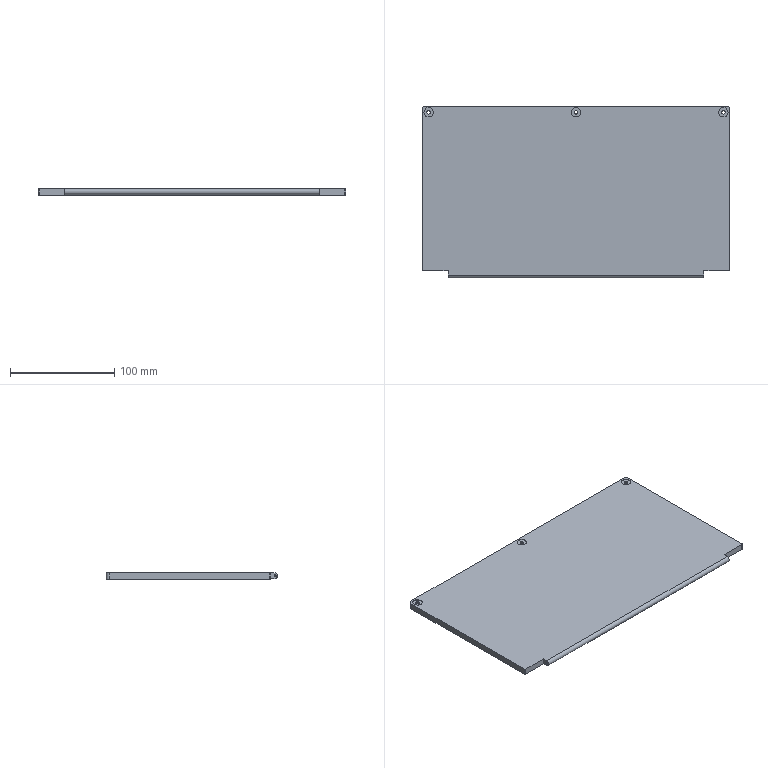NC program | Mastercam | posted with a generic post
Lines 868 to 1870 of 5159:
N8670 T6 M6
N8680 G0 G90 G17 G54 X-57.409 Y78.94 A0. S7000 M3
N8690 G43 H6 Z50. M8
N8700 Z1.
N8710 G1 Z.225 F600.
N8720 X-54.109 Z.123 F3000.
N8730 X-50.809 Z.021
N8740 X-47.509 Z-.08
N8750 X-44.209 Z-.182
N8760 X-40.909 Z-.284
N8770 X-37.609 Z-.386
N8780 X-32.744 Z-.487
N8790 G2 X-32.455 Y79.06 I27.577 J-66.293
N8800 G1 X-34.311
N8810 X-50.628
N8820 X-68.56
N8830 Y78.94
N8840 X-32.744
N8850 G2 X-32.455 Y79.06 I27.577 J-66.293
N8860 G1 X-34.311
N8870 G2 X-34.897 Y79.479 I0. J.618
N8880 G1 X-35.581 Y81.494
N8890 G3 X-36.167 Y81.913 I-.586 J-.2
N8900 G1 X-50.628
N8910 X-71.413
N8920 Y76.087
N8930 X-32.168
N8940 G2 X-7.749 Y81.913 I30.414 J-73.385
N8950 G1 X-36.167
N8960 G0 Z50.
N8970 X57.411 Y79.06
N8980 Z1.
N8990 G1 Z.225 F600.
N9000 X54.111 Z.123 F3000.
N9010 X50.811 Z.021
N9020 X47.511 Z-.08
N9030 X44.211 Z-.182
N9040 X40.911 Z-.284
N9050 X37.611 Z-.386
N9060 X32.455 Z-.487
N9070 X34.311 Y79.048
N9080 X50.628 Y78.94
N9090 X68.56
N9100 Y79.06
N9110 X32.455
N9120 X34.311 Y79.048
N9130 X34.315
N9140 G3 X34.933 Y79.666 I0. J.618
N9150 X34.723 Y80.132 I-.618 J0.
N9160 G1 X32.862 Y81.76
N9170 G3 X32.455 Y81.913 I-.407 J-.466
N9180 G1 X7.749
N9190 G2 X32.168 Y76.087 I-5.995 J-79.211
N9200 G1 X50.628
N9210 X71.413
N9220 Y81.913
N9230 X32.455
N9240 G2 X31.881 Y82.3 I0. J.619
N9250 G1 X31.172 Y84.056
N9260 G3 X30.599 Y84.443 I-.573 J-.232
N9270 G1 X0.
N9280 X-73.943
N9290 Y73.557
N9300 X-31.647
N9310 G2 X-1.474 Y79.656 I30.173 J-71.581
N9320 X2.458 Y79.557 I0. J-77.68
N9330 X31.647 Y73.557 I-.115 J-74.561
N9340 G1 X73.943
N9350 Y84.443
N9360 X30.599
N9370 G2 X29.994 Y84.928 I0. J.619
N9380 G1 X29.347 Y87.865
N9390 G3 X28.742 Y88.35 I-.605 J-.134
N9400 G1 X0.
N9410 X-77.85
N9420 Y69.65
N9430 X-30.822
N9440 G2 X-1.437 Y75.753 I29.385 J-67.691
N9450 X2.458 Y75.65 I0. J-73.794
N9460 X30.822 Y69.65 I-.108 J-70.552
N9470 G1 X77.85
N9480 Y88.35
N9490 X28.742
N9500 G2 X28.138 Y88.835 I0. J.619
N9510 G1 X27.49 Y91.772
N9520 G3 X26.886 Y92.257 I-.604 J-.134
N9530 G1 X0.
N9540 X-81.757
N9550 Y65.743
N9560 X-29.97
N9570 G2 X-1.396 Y71.849 I28.574 J-63.801
N9580 X2.458 Y71.743 I0. J-69.907
N9590 X29.97 Y65.743 I-.099 J-66.53
N9600 G1 X81.757
N9610 Y92.257
N9620 X26.886
N9630 G2 X26.282 Y92.742 I0. J.619
N9640 G1 X25.634 Y95.678
N9650 G3 X25.03 Y96.164 I-.604 J-.133
N9660 G1 X0.
N9670 X-85.664
N9680 Y61.836
N9690 X-29.088
N9700 G2 X-1.371 Y67.948 I27.717 J-59.793
N9710 X2.458 Y67.836 I0. J-65.905
N9720 X29.088 Y61.836 I-.089 J-62.489
N9730 G1 X85.664
N9740 Y96.164
N9750 X25.03
N9760 G2 X24.426 Y96.649 I0. J.618
N9770 G1 X23.778 Y99.585
N9780 G3 X23.174 Y100.07 I-.604 J-.133
N9790 G1 X0.
N9800 X-89.57
N9810 Y57.93
N9820 X-28.171
N9830 G2 X-1.357 Y64.048 I26.814 J-55.705
N9840 X2.458 Y63.93 I0. J-61.823
N9850 X28.171 Y57.93 I-.044 J-58.289
N9860 G1 X89.57
N9870 Y100.07
N9880 X23.174
N9890 G2 X22.569 Y100.556 I0. J.619
N9900 G1 X21.922 Y103.492
N9910 G3 X21.317 Y103.977 I-.605 J-.133
N9920 G1 X0.
N9930 X-93.477
N9940 Y54.023
N9950 X-27.222
N9960 G2 X-1.331 Y60.148 I25.891 J-51.663
N9970 X2.458 Y60.023 I0. J-57.788
N9980 X27.222 Y54.023 I-.007 J-54.13
N9990 G1 X93.477
N100 Y103.977
N110 X21.317
N120 G2 X20.713 Y104.463 I0. J.619
N130 G1 X20.065 Y107.399
N140 G3 X19.461 Y107.884 I-.604 J-.134
N150 G1 X0.
N160 X-97.384
N170 Y50.116
N180 X-26.251
N190 G2 X-1.291 Y56.246 I24.96 J-47.748
N200 X2.458 Y56.116 I0. J-53.878
N210 G1 X2.463
N220 G2 X26.251 Y50.116 I0. J-50.159
N230 G1 X97.384
N240 Y107.884
N250 X19.461
N260 G2 X18.857 Y108.369 I0. J.619
N270 G1 X18.209 Y111.306
N280 G3 X17.605 Y111.791 I-.604 J-.134
N290 G1 X0.
N300 X-101.291
N310 Y46.209
N320 X-25.233
N330 G2 X-1.247 Y52.346 I23.986 J-43.802
N340 X2.458 Y52.209 I0. J-49.939
N350 G1 X2.479
N360 G2 X25.233 Y46.209 I0. J-46.148
N370 G1 X101.291
N380 Y111.791
N390 X17.605
N400 G2 X17.001 Y112.276 I0. J.619
N410 G1 X16.353 Y115.212
N420 G3 X15.749 Y115.698 I-.604 J-.133
N430 G1 X0.
N440 X-105.198
N450 Y42.302
N460 X-24.182
N470 G2 X-1.192 Y48.447 I22.99 J-39.935
N480 X2.458 Y48.302 I0. J-46.08
N490 G1 X2.476
N500 G2 X24.182 Y42.302 I0. J-42.263
N510 G1 X105.198
N520 Y115.698
N530 X15.749
N540 G2 X15.144 Y116.183 I0. J.619
N550 G1 X14.497 Y119.119
N560 G3 X13.892 Y119.605 I-.605 J-.133
N570 G1 X0.
N580 X-109.105
N590 Y38.395
N600 X-23.072
N610 G2 X-1.134 Y44.548 I21.938 J-36.03
N620 X2.458 Y44.395 I0. J-42.183
N630 G1 X2.476
N640 G2 X23.072 Y38.395 I0. J-38.347
N650 G1 X109.105
N660 Y119.605
N670 X13.892
N680 G2 X13.288 Y120.09 I0. J.618
N690 G1 X12.64 Y123.026
N700 G3 X12.036 Y123.512 I-.604 J-.133
N710 G1 X0.
N720 X-113.012
N730 Y34.488
N740 X-21.883
N750 G2 X-2.16 Y40.554 I19.723 J-29.028
N760 X0. Y40.488 I0. J-35.094
N770 X2.16 Y40.555 I2.16 J-35.028
N780 X21.883 Y34.488 I0. J-35.095
N790 G1 X113.012
N800 Y123.512
N810 X12.036
N820 G2 X11.432 Y123.997 I0. J.618
N830 G1 X10.784 Y126.933
N840 G3 X10.18 Y127.419 I-.604 J-.133
N850 G1 X0.
N860 X-116.919
N870 Y30.581
N880 X-20.606
N890 G2 X-1.052 Y36.763 I19.554 J-27.836
N900 X2.458 Y36.581 I0. J-34.018
N910 G1 X2.521
N920 G2 X20.606 Y30.581 I0. J-30.256
N930 G1 X116.919
N940 Y127.419
N950 X10.18
N960 G2 X9.576 Y127.904 I0. J.618
N970 G1 X8.928 Y130.84
N980 G3 X8.324 Y131.325 I-.604 J-.133
N990 G1 X0.
N1000 X-120.825
N1010 Y26.675
N1020 X-19.231
N1030 G2 X-9.646 Y31.72 I18.178 J-22.906
N1040 X.06 Y32.736 I9.706 J-45.863
N1050 X2.458 Y32.675 I0. J-46.879
N1060 G1 X2.569
N1070 G2 X19.231 Y26.675 I0. J-26.136
N1080 G1 X120.825
N1090 Y131.325
N1100 X8.324
N1110 G2 X7.719 Y131.811 I0. J.619
N1120 G1 X7.072 Y134.747
N1130 G3 X6.467 Y135.232 I-.605 J-.133
N1140 G1 X0.
N1150 X-124.732
N1160 Y22.768
N1170 X-17.749
N1180 G2 X-9.083 Y27.812 I16.408 J-18.221
N1190 X.033 Y28.839 I9.116 J-39.926
N1200 X2.458 Y28.768 I0. J-40.953
N1210 G1 X2.602
N1220 G2 X17.749 Y22.768 I0. J-22.118
N1230 G1 X124.732
N1240 Y135.232
N1250 X6.467
N1260 G2 X5.863 Y135.718 I0. J.619
N1270 G1 X5.215 Y138.654
N1280 G3 X4.611 Y139.139 I-.604 J-.133
N1290 G1 X0.
N1300 X-128.639
N1310 Y20.156
N1320 X-127.344 Y18.861
N1330 X-16.156
N1340 G2 X-8.479 Y23.904 I14.872 J-14.274
N1350 X.017 Y24.946 I8.496 J-34.117
N1360 X2.458 Y24.861 I0. J-35.159
N1370 G1 X2.569
N1380 G2 X16.156 Y18.861 I0. J-18.382
N1390 G1 X127.344
N1400 X128.639 Y20.156
N1410 Y139.139
N1420 X4.611
N1430 G2 X4.007 Y139.625 I0. J.619
N1440 G1 X3.359 Y142.561
N1450 G3 X2.755 Y143.046 I-.604 J-.134
N1460 G1 X0.
N1470 X-132.546
N1480 Y18.537
N1490 X-128.963 Y14.954
N1500 X-14.537
N1510 G2 X-7.724 Y20.031 I15.103 J-13.158
N1520 X.111 Y21.055 I7.835 J-29.465
N1530 X2.604 Y20.953 I0. J-30.489
N1540 X14.537 Y14.954 I-.387 J-15.639
N1550 G1 X128.963
N1560 X132.546 Y18.537
N1570 Y143.046
N1580 X2.755
N1590 G2 X2.151 Y143.532 I0. J.619
N1600 G1 X1.503 Y146.468
N1610 G3 X.899 Y146.953 I-.604 J-.134
N1620 G1 X0.
N1630 X-136.453
N1640 Y16.919
N1650 X-130.581 Y11.047
N1660 X-12.919
N1670 G2 X-6.446 Y16.339 I16.004 J-12.971
N1680 X.1 Y17.151 I6.546 J-25.972
N1690 X2.458 Y17.047 I0. J-26.784
N1700 X7.68 Y15.742 I-.48 J-13.021
N1710 X12.919 Y11.047 I-12.589 J-19.319
N1720 G1 X130.581
N1730 X136.453 Y16.919
N1740 Y146.953
N1750 X.899
N1760 G2 X.28 Y147.572 I0. J.619
N1770 X.285 Y147.652 I.619 J0.
N1780 G1 X.614 Y150.161
N1790 G3 X.619 Y150.241 I-.614 J.08
N1800 X0. Y150.86 I-.619 J0.
N1810 G1 X-140.244
N1820 X-140.353 Y150.853
N1830 X-140.36 Y150.268
N1840 Y15.924
N1850 X-140.343 Y15.309
N1860 X-140.261 Y15.202
N1870 X-132.474 Y7.414
N1880 X-132.193 Y7.158
N1890 X-132.081 Y7.143
N1900 X-131.927 Y7.14
N1910 X-11.506
N1920 X-11.309 Y7.157
N1930 X-11.199 Y7.242
N1940 X-6.862 Y11.555
N1950 G2 X-5.167 Y12.647 I4.319 J-4.842
N1960 X-3.005 Y13.13 I2.491 J-6.075
N1970 X.043 Y13.157 I3.048 J-169.278
N1980 X2.458 Y13.14 I0. J-169.305
N1990 X2.676 Y13.144 I.218 J-6.388
N2000 X6.175 Y12.101 I0. J-6.392
N2010 X7.375 Y11.066 I-7.862 J-10.326
N2020 G1 X11.199 Y7.242
N2030 X11.309 Y7.157
N2040 X11.506 Y7.14
N2050 X131.927
N2060 X132.193 Y7.158
N2070 X132.474 Y7.414
N2080 X140.261 Y15.202
N2090 X140.342 Y15.307
N2100 X140.352 Y15.378
N2110 X140.36 Y150.268
N2120 X140.354 Y150.85
N2130 X140.244 Y150.86
N2140 X0.
N2150 G0 Z50.
N2160 X-57.409 Y78.94
N2170 Z.512
N2180 G1 Z-.263 F600.
N2190 X-54.109 Z-.364 F3000.
N2200 X-50.809 Z-.466
N2210 X-47.509 Z-.568
N2220 X-44.209 Z-.67
N2230 X-40.909 Z-.771
N2240 X-37.609 Z-.873
N2250 X-32.744 Z-.975
N2260 G2 X-32.455 Y79.06 I27.577 J-66.293
N2270 G1 X-34.311
N2280 X-50.628
N2290 X-68.56
N2300 Y78.94
N2310 X-32.744
N2320 G2 X-32.455 Y79.06 I27.577 J-66.293
N2330 G1 X-34.311
N2340 G2 X-34.897 Y79.479 I0. J.618
N2350 G1 X-35.581 Y81.494
N2360 G3 X-36.167 Y81.913 I-.586 J-.2
N2370 G1 X-50.628
N2380 X-71.413
N2390 Y76.087
N2400 X-32.168
N2410 G2 X-7.749 Y81.913 I30.414 J-73.385
N2420 G1 X-36.167
N2430 G0 Z50.
N2440 X57.411 Y79.06
N2450 Z.512
N2460 G1 Z-.263 F600.
N2470 X54.111 Z-.364 F3000.
N2480 X50.811 Z-.466
N2490 X47.511 Z-.568
N2500 X44.211 Z-.67
N2510 X40.911 Z-.771
N2520 X37.611 Z-.873
N2530 X32.455 Z-.975
N2540 X34.311 Y79.048
N2550 X50.628 Y78.94
N2560 X68.56
N2570 Y79.06
N2580 X32.455
N2590 X34.311 Y79.048
N2600 X34.315
N2610 G3 X34.933 Y79.666 I0. J.618
N2620 X34.723 Y80.132 I-.618 J0.
N2630 G1 X32.862 Y81.76
N2640 G3 X32.455 Y81.913 I-.407 J-.466
N2650 G1 X7.749
N2660 G2 X32.168 Y76.087 I-5.995 J-79.211
N2670 G1 X50.628
N2680 X71.413
N2690 Y81.913
N2700 X32.455
N2710 G2 X31.881 Y82.3 I0. J.619
N2720 G1 X31.172 Y84.056
N2730 G3 X30.599 Y84.443 I-.573 J-.232
N2740 G1 X0.
N2750 X-73.943
N2760 Y73.557
N2770 X-31.647
N2780 G2 X-1.474 Y79.656 I30.173 J-71.581
N2790 X2.458 Y79.557 I0. J-77.68
N2800 X31.647 Y73.557 I-.115 J-74.561
N2810 G1 X73.943
N2820 Y84.443
N2830 X30.599
N2840 G2 X29.994 Y84.928 I0. J.619
N2850 G1 X29.347 Y87.865
N2860 G3 X28.742 Y88.35 I-.605 J-.134
N2870 G1 X0.
N2880 X-77.85
N2890 Y69.65
N2900 X-30.822
N2910 G2 X-1.437 Y75.753 I29.385 J-67.691
N2920 X2.458 Y75.65 I0. J-73.794
N2930 X30.822 Y69.65 I-.108 J-70.552
N2940 G1 X77.85
N2950 Y88.35
N2960 X28.742
N2970 G2 X28.138 Y88.835 I0. J.619
N2980 G1 X27.49 Y91.772
N2990 G3 X26.886 Y92.257 I-.604 J-.134
N3000 G1 X0.
N3010 X-81.757
N3020 Y65.743
N3030 X-29.97
N3040 G2 X-1.396 Y71.849 I28.574 J-63.801
N3050 X2.458 Y71.743 I0. J-69.907
N3060 X29.97 Y65.743 I-.099 J-66.53
N3070 G1 X81.757
N3080 Y92.257
N3090 X26.886
N3100 G2 X26.282 Y92.742 I0. J.619
N3110 G1 X25.634 Y95.678
N3120 G3 X25.03 Y96.164 I-.604 J-.133
N3130 G1 X0.
N3140 X-85.664
N3150 Y61.836
N3160 X-29.088
N3170 G2 X-1.371 Y67.948 I27.717 J-59.793
N3180 X2.458 Y67.836 I0. J-65.905
N3190 X29.088 Y61.836 I-.089 J-62.489
N3200 G1 X85.664
N3210 Y96.164
N3220 X25.03
N3230 G2 X24.426 Y96.649 I0. J.618
N3240 G1 X23.778 Y99.585
N3250 G3 X23.174 Y100.07 I-.604 J-.133
N3260 G1 X0.
N3270 X-89.57
N3280 Y57.93
N3290 X-28.171
N3300 G2 X-1.357 Y64.048 I26.814 J-55.705
N3310 X2.458 Y63.93 I0. J-61.823
N3320 X28.171 Y57.93 I-.044 J-58.289
N3330 G1 X89.57
N3340 Y100.07
N3350 X23.174
N3360 G2 X22.569 Y100.556 I0. J.619
N3370 G1 X21.922 Y103.492
N3380 G3 X21.317 Y103.977 I-.605 J-.133
N3390 G1 X0.
N3400 X-93.477
N3410 Y54.023
N3420 X-27.222
N3430 G2 X-1.331 Y60.148 I25.891 J-51.663
N3440 X2.458 Y60.023 I0. J-57.788
N3450 X27.222 Y54.023 I-.007 J-54.13
N3460 G1 X93.477
N3470 Y103.977
N3480 X21.317
N3490 G2 X20.713 Y104.463 I0. J.619
N3500 G1 X20.065 Y107.399
N3510 G3 X19.461 Y107.884 I-.604 J-.134
N3520 G1 X0.
N3530 X-97.384
N3540 Y50.116
N3550 X-26.251
N3560 G2 X-1.291 Y56.246 I24.96 J-47.748
N3570 X2.458 Y56.116 I0. J-53.878
N3580 G1 X2.463
N3590 G2 X26.251 Y50.116 I0. J-50.159
N3600 G1 X97.384
N3610 Y107.884
N3620 X19.461
N3630 G2 X18.857 Y108.369 I0. J.619
N3640 G1 X18.209 Y111.306
N3650 G3 X17.605 Y111.791 I-.604 J-.134
N3660 G1 X0.
N3670 X-101.291
N3680 Y46.209
N3690 X-25.233
N3700 G2 X-1.247 Y52.346 I23.986 J-43.802
N3710 X2.458 Y52.209 I0. J-49.939
N3720 G1 X2.479
N3730 G2 X25.233 Y46.209 I0. J-46.148
N3740 G1 X101.291
N3750 Y111.791
N3760 X17.605
N3770 G2 X17.001 Y112.276 I0. J.619
N3780 G1 X16.353 Y115.212
N3790 G3 X15.749 Y115.698 I-.604 J-.133
N3800 G1 X0.
N3810 X-105.198
N3820 Y42.302
N3830 X-24.182
N3840 G2 X-1.192 Y48.447 I22.99 J-39.935
N3850 X2.458 Y48.302 I0. J-46.08
N3860 G1 X2.476
N3870 G2 X24.182 Y42.302 I0. J-42.263
N3880 G1 X105.198
N3890 Y115.698
N3900 X15.749
N3910 G2 X15.144 Y116.183 I0. J.619
N3920 G1 X14.497 Y119.119
N3930 G3 X13.892 Y119.605 I-.605 J-.133
N3940 G1 X0.
N3950 X-109.105
N3960 Y38.395
N3970 X-23.072
N3980 G2 X-1.134 Y44.548 I21.938 J-36.03
N3990 X2.458 Y44.395 I0. J-42.183
N4000 G1 X2.476
N4010 G2 X23.072 Y38.395 I0. J-38.347
N4020 G1 X109.105
N4030 Y119.605
N4040 X13.892
N4050 G2 X13.288 Y120.09 I0. J.618
N4060 G1 X12.64 Y123.026
N4070 G3 X12.036 Y123.512 I-.604 J-.133
N4080 G1 X0.
N4090 X-113.012
N4100 Y34.488
N4110 X-21.883
N4120 G2 X-2.16 Y40.554 I19.723 J-29.028
N4130 X0. Y40.488 I0. J-35.094
N4140 X2.16 Y40.555 I2.16 J-35.028
N4150 X21.883 Y34.488 I0. J-35.095
N4160 G1 X113.012
N4170 Y123.512
N4180 X12.036
N4190 G2 X11.432 Y123.997 I0. J.618
N4200 G1 X10.784 Y126.933
N4210 G3 X10.18 Y127.419 I-.604 J-.133
N4220 G1 X0.
N4230 X-116.919
N4240 Y30.581
N4250 X-20.606
N4260 G2 X-1.052 Y36.763 I19.554 J-27.836
N4270 X2.458 Y36.581 I0. J-34.018
N4280 G1 X2.521
N4290 G2 X20.606 Y30.581 I0. J-30.256
N4300 G1 X116.919
N4310 Y127.419
N4320 X10.18
N4330 G2 X9.576 Y127.904 I0. J.618
N4340 G1 X8.928 Y130.84
N4350 G3 X8.324 Y131.325 I-.604 J-.133
N4360 G1 X0.
N4370 X-120.825
N4380 Y26.675
N4390 X-19.231
N4400 G2 X-9.646 Y31.72 I18.178 J-22.906
N4410 X.06 Y32.736 I9.706 J-45.863
N4420 X2.458 Y32.675 I0. J-46.879
N4430 G1 X2.569
N4440 G2 X19.231 Y26.675 I0. J-26.136
N4450 G1 X120.825
N4460 Y131.325
N4470 X8.324
N4480 G2 X7.719 Y131.811 I0. J.619
N4490 G1 X7.072 Y134.747
N4500 G3 X6.467 Y135.232 I-.605 J-.133
N4510 G1 X0.
N4520 X-124.732
N4530 Y22.768
N4540 X-17.749
N4550 G2 X-9.083 Y27.812 I16.408 J-18.221
N4560 X.033 Y28.839 I9.116 J-39.926
N4570 X2.458 Y28.768 I0. J-40.953
N4580 G1 X2.602
N4590 G2 X17.749 Y22.768 I0. J-22.118
N4600 G1 X124.732
N4610 Y135.232
N4620 X6.467
N4630 G2 X5.863 Y135.718 I0. J.619
N4640 G1 X5.215 Y138.654
N4650 G3 X4.611 Y139.139 I-.604 J-.133
N4660 G1 X0.
N4670 X-128.639
N4680 Y20.156
N4690 X-127.344 Y18.861
N4700 X-16.156
N4710 G2 X-8.479 Y23.904 I14.872 J-14.274
N4720 X.017 Y24.946 I8.496 J-34.117
N4730 X2.458 Y24.861 I0. J-35.159
N4740 G1 X2.569
N4750 G2 X16.156 Y18.861 I0. J-18.382
N4760 G1 X127.344
N4770 X128.639 Y20.156
N4780 Y139.139
N4790 X4.611
N4800 G2 X4.007 Y139.625 I0. J.619
N4810 G1 X3.359 Y142.561
N4820 G3 X2.755 Y143.046 I-.604 J-.134
N4830 G1 X0.
N4840 X-132.546
N4850 Y18.537
N4860 X-128.963 Y14.954
N4870 X-14.537
N4880 G2 X-7.724 Y20.031 I15.103 J-13.158
N4890 X.111 Y21.055 I7.835 J-29.465
N4900 X2.604 Y20.953 I0. J-30.489
N4910 X14.537 Y14.954 I-.387 J-15.639
N4920 G1 X128.963
N4930 X132.546 Y18.537
N4940 Y143.046
N4950 X2.755
N4960 G2 X2.151 Y143.532 I0. J.619
N4970 G1 X1.503 Y146.468
N4980 G3 X.899 Y146.953 I-.604 J-.134
N4990 G1 X0.
N5000 X-136.453
N5010 Y16.919
N5020 X-130.581 Y11.047
N5030 X-12.919
N5040 G2 X-6.446 Y16.339 I16.004 J-12.971
N5050 X.1 Y17.151 I6.546 J-25.972
N5060 X2.458 Y17.047 I0. J-26.784
N5070 X7.68 Y15.742 I-.48 J-13.021
N5080 X12.919 Y11.047 I-12.589 J-19.319
N5090 G1 X130.581
N5100 X136.453 Y16.919
N5110 Y146.953
N5120 X.899
N5130 G2 X.28 Y147.572 I0. J.619
N5140 X.285 Y147.652 I.619 J0.
N5150 G1 X.614 Y150.161
N5160 G3 X.619 Y150.241 I-.614 J.08
N5170 X0. Y150.86 I-.619 J0.
N5180 G1 X-140.244
N5190 X-140.353 Y150.853
N5200 X-140.36 Y150.268
N5210 Y15.924
N5220 X-140.343 Y15.309
N5230 X-140.261 Y15.202
N5240 X-132.474 Y7.414
N5250 X-132.193 Y7.158
N5260 X-132.081 Y7.143
N5270 X-131.927 Y7.14
N5280 X-11.506
N5290 X-11.309 Y7.157
N5300 X-11.199 Y7.242
N5310 X-6.862 Y11.555
N5320 G2 X-5.167 Y12.647 I4.319 J-4.842
N5330 X-3.005 Y13.13 I2.491 J-6.075
N5340 X.043 Y13.157 I3.048 J-169.278
N5350 X2.458 Y13.14 I0. J-169.305
N5360 X2.676 Y13.144 I.218 J-6.388
N5370 X6.175 Y12.101 I0. J-6.392
N5380 X7.375 Y11.066 I-7.862 J-10.326
N5390 G1 X11.199 Y7.242
N5400 X11.309 Y7.157
N5410 X11.506 Y7.14
N5420 X131.927
N5430 X132.193 Y7.158
N5440 X132.474 Y7.414
N5450 X140.261 Y15.202
N5460 X140.342 Y15.307
N5470 X140.352 Y15.378
N5480 X140.36 Y150.268
N5490 X140.354 Y150.85
N5500 X140.244 Y150.86
N5510 X0.
N5520 G0 Z50.
N5530 X-57.409 Y78.94
N5540 Z.025
N5550 G1 Z-.75 F600.
N5560 X-54.109 Z-.852 F3000.
N5570 X-50.809 Z-.954
N5580 X-47.509 Z-1.055
N5590 X-44.209 Z-1.157
N5600 X-40.909 Z-1.259
N5610 X-37.609 Z-1.361
N5620 X-32.744 Z-1.462
N5630 G2 X-32.455 Y79.06 I27.577 J-66.293
N5640 G1 X-34.311
N5650 X-50.628
N5660 X-68.56
N5670 Y78.94
N5680 X-32.744
N5690 G2 X-32.455 Y79.06 I27.577 J-66.293
N5700 G1 X-34.311
N5710 G2 X-34.897 Y79.479 I0. J.618
N5720 G1 X-35.581 Y81.494
N5730 G3 X-36.167 Y81.913 I-.586 J-.2
N5740 G1 X-50.628
N5750 X-71.413
N5760 Y76.087
N5770 X-32.168
N5780 G2 X-7.749 Y81.913 I30.414 J-73.385
N5790 G1 X-36.167
N5800 G0 Z50.
N5810 X57.411 Y79.06
N5820 Z.025
N5830 G1 Z-.75 F600.
N5840 X54.111 Z-.852 F3000.
N5850 X50.811 Z-.954
N5860 X47.511 Z-1.055
N5870 X44.211 Z-1.157
N5880 X40.911 Z-1.259
N5890 X37.611 Z-1.361
N5900 X32.455 Z-1.462
N5910 X34.311 Y79.048
N5920 X50.628 Y78.94
N5930 X68.56
N5940 Y79.06
N5950 X32.455
N5960 X34.311 Y79.048
N5970 X34.315
N5980 G3 X34.933 Y79.666 I0. J.618
N5990 X34.723 Y80.132 I-.618 J0.
N6000 G1 X32.862 Y81.76
N6010 G3 X32.455 Y81.913 I-.407 J-.466
N6020 G1 X7.749
N6030 G2 X32.168 Y76.087 I-5.995 J-79.211
N6040 G1 X50.628
N6050 X71.413
N6060 Y81.913
N6070 X32.455
N6080 G2 X31.881 Y82.3 I0. J.619
N6090 G1 X31.172 Y84.056
N6100 G3 X30.599 Y84.443 I-.573 J-.232
N6110 G1 X0.
N6120 X-73.943
N6130 Y73.557
N6140 X-31.647
N6150 G2 X-1.474 Y79.656 I30.173 J-71.581
N6160 X2.458 Y79.557 I0. J-77.68
N6170 X31.647 Y73.557 I-.115 J-74.561
N6180 G1 X73.943
N6190 Y84.443
N6200 X30.599
N6210 G2 X29.994 Y84.928 I0. J.619
N6220 G1 X29.347 Y87.865
N6230 G3 X28.742 Y88.35 I-.605 J-.134
N6240 G1 X0.
N6250 X-77.85
N6260 Y69.65
N6270 X-30.822
N6280 G2 X-1.437 Y75.753 I29.385 J-67.691
N6290 X2.458 Y75.65 I0. J-73.794
N6300 X30.822 Y69.65 I-.108 J-70.552
N6310 G1 X77.85
N6320 Y88.35
N6330 X28.742
N6340 G2 X28.138 Y88.835 I0. J.619
N6350 G1 X27.49 Y91.772
N6360 G3 X26.886 Y92.257 I-.604 J-.134
N6370 G1 X0.
N6380 X-81.757
N6390 Y65.743
N6400 X-29.97
N6410 G2 X-1.396 Y71.849 I28.574 J-63.801
N6420 X2.458 Y71.743 I0. J-69.907
N6430 X29.97 Y65.743 I-.099 J-66.53
N6440 G1 X81.757
N6450 Y92.257
N6460 X26.886
N6470 G2 X26.282 Y92.742 I0. J.619
N6480 G1 X25.634 Y95.678
N6490 G3 X25.03 Y96.164 I-.604 J-.133
N6500 G1 X0.
N6510 X-85.664
N6520 Y61.836
N6530 X-29.088
N6540 G2 X-1.371 Y67.948 I27.717 J-59.793
N6550 X2.458 Y67.836 I0. J-65.905
N6560 X29.088 Y61.836 I-.089 J-62.489
N6570 G1 X85.664
N6580 Y96.164
N6590 X25.03
N6600 G2 X24.426 Y96.649 I0. J.618
N6610 G1 X23.778 Y99.585
N6620 G3 X23.174 Y100.07 I-.604 J-.133
N6630 G1 X0.
N6640 X-89.57
N6650 Y57.93
N6660 X-28.171
N6670 G2 X-1.357 Y64.048 I26.814 J-55.705
N6680 X2.458 Y63.93 I0. J-61.823
N6690 X28.171 Y57.93 I-.044 J-58.289
N6700 G1 X89.57
N6710 Y100.07
N6720 X23.174
N6730 G2 X22.569 Y100.556 I0. J.619
N6740 G1 X21.922 Y103.492
N6750 G3 X21.317 Y103.977 I-.605 J-.133
N6760 G1 X0.
N6770 X-93.477
N6780 Y54.023
N6790 X-27.222
N6800 G2 X-1.331 Y60.148 I25.891 J-51.663
N6810 X2.458 Y60.023 I0. J-57.788
N6820 X27.222 Y54.023 I-.007 J-54.13
N6830 G1 X93.477
N6840 Y103.977
N6850 X21.317
N6860 G2 X20.713 Y104.463 I0. J.619
N6870 G1 X20.065 Y107.399
N6880 G3 X19.461 Y107.884 I-.604 J-.134
N6890 G1 X0.
N6900 X-97.384
N6910 Y50.116
N6920 X-26.251
N6930 G2 X-1.291 Y56.246 I24.96 J-47.748
N6940 X2.458 Y56.116 I0. J-53.878
N6950 G1 X2.463
N6960 G2 X26.251 Y50.116 I0. J-50.159
N6970 G1 X97.384
N6980 Y107.884
N6990 X19.461
N7000 G2 X18.857 Y108.369 I0. J.619
N7010 G1 X18.209 Y111.306
N7020 G3 X17.605 Y111.791 I-.604 J-.134
N7030 G1 X0.
N7040 X-101.291
N7050 Y46.209
N7060 X-25.233
N7070 G2 X-1.247 Y52.346 I23.986 J-43.802
N7080 X2.458 Y52.209 I0. J-49.939
N7090 G1 X2.479
N7100 G2 X25.233 Y46.209 I0. J-46.148
N7110 G1 X101.291
N7120 Y111.791
N7130 X17.605
N7140 G2 X17.001 Y112.276 I0. J.619
N7150 G1 X16.353 Y115.212
N7160 G3 X15.749 Y115.698 I-.604 J-.133
N7170 G1 X0.
N7180 X-105.198
N7190 Y42.302
N7200 X-24.182
N7210 G2 X-1.192 Y48.447 I22.99 J-39.935
N7220 X2.458 Y48.302 I0. J-46.08
N7230 G1 X2.476
N7240 G2 X24.182 Y42.302 I0. J-42.263
N7250 G1 X105.198
N7260 Y115.698
N7270 X15.749
N7280 G2 X15.144 Y116.183 I0. J.619
N7290 G1 X14.497 Y119.119
N7300 G3 X13.892 Y119.605 I-.605 J-.133
N7310 G1 X0.
N7320 X-109.105
N7330 Y38.395
N7340 X-23.072
N7350 G2 X-1.134 Y44.548 I21.938 J-36.03
N7360 X2.458 Y44.395 I0. J-42.183
N7370 G1 X2.476
N7380 G2 X23.072 Y38.395 I0. J-38.347
N7390 G1 X109.105
N7400 Y119.605
N7410 X13.892
N7420 G2 X13.288 Y120.09 I0. J.618
N7430 G1 X12.64 Y123.026
N7440 G3 X12.036 Y123.512 I-.604 J-.133
N7450 G1 X0.
N7460 X-113.012
N7470 Y34.488
N7480 X-21.883
N7490 G2 X-2.16 Y40.554 I19.723 J-29.028
N7500 X0. Y40.488 I0. J-35.094
N7510 X2.16 Y40.555 I2.16 J-35.028
N7520 X21.883 Y34.488 I0. J-35.095
N7530 G1 X113.012
N7540 Y123.512
N7550 X12.036
N7560 G2 X11.432 Y123.997 I0. J.618
N7570 G1 X10.784 Y126.933
N7580 G3 X10.18 Y127.419 I-.604 J-.133
N7590 G1 X0.
N7600 X-116.919
N7610 Y30.581
N7620 X-20.606
N7630 G2 X-1.052 Y36.763 I19.554 J-27.836
N7640 X2.458 Y36.581 I0. J-34.018
N7650 G1 X2.521
N7660 G2 X20.606 Y30.581 I0. J-30.256
N7670 G1 X116.919
N7680 Y127.419
N7690 X10.18
N7700 G2 X9.576 Y127.904 I0. J.618
N7710 G1 X8.928 Y130.84
N7720 G3 X8.324 Y131.325 I-.604 J-.133
N7730 G1 X0.
N7740 X-120.825
N7750 Y26.675
N7760 X-19.231
N7770 G2 X-9.646 Y31.72 I18.178 J-22.906
N7780 X.06 Y32.736 I9.706 J-45.863
N7790 X2.458 Y32.675 I0. J-46.879
N7800 G1 X2.569
N7810 G2 X19.231 Y26.675 I0. J-26.136
N7820 G1 X120.825
N7830 Y131.325
N7840 X8.324
N7850 G2 X7.719 Y131.811 I0. J.619
N7860 G1 X7.072 Y134.747
N7870 G3 X6.467 Y135.232 I-.605 J-.133
N7880 G1 X0.
N7890 X-124.732
N7900 Y22.768
N7910 X-17.749
N7920 G2 X-9.083 Y27.812 I16.408 J-18.221
N7930 X.033 Y28.839 I9.116 J-39.926
N7940 X2.458 Y28.768 I0. J-40.953
N7950 G1 X2.602
N7960 G2 X17.749 Y22.768 I0. J-22.118
N7970 G1 X124.732
N7980 Y135.232
N7990 X6.467
N8000 G2 X5.863 Y135.718 I0. J.619
N8010 G1 X5.215 Y138.654
N8020 G3 X4.611 Y139.139 I-.604 J-.133
N8030 G1 X0.
N8040 X-128.639
N8050 Y20.156
N8060 X-127.344 Y18.861
N8070 X-16.156
N8080 G2 X-8.479 Y23.904 I14.872 J-14.274
N8090 X.017 Y24.946 I8.496 J-34.117
N8100 X2.458 Y24.861 I0. J-35.159
N8110 G1 X2.569
N8120 G2 X16.156 Y18.861 I0. J-18.382
N8130 G1 X127.344
N8140 X128.639 Y20.156
N8150 Y139.139
N8160 X4.611
N8170 G2 X4.007 Y139.625 I0. J.619
N8180 G1 X3.359 Y142.561
N8190 G3 X2.755 Y143.046 I-.604 J-.134
N8200 G1 X0.
N8210 X-132.546
N8220 Y18.537
N8230 X-128.963 Y14.954
N8240 X-14.537
N8250 G2 X-7.724 Y20.031 I15.103 J-13.158
N8260 X.111 Y21.055 I7.835 J-29.465
N8270 X2.604 Y20.953 I0. J-30.489
N8280 X14.537 Y14.954 I-.387 J-15.639
N8290 G1 X128.963
N8300 X132.546 Y18.537
N8310 Y143.046
N8320 X2.755
N8330 G2 X2.151 Y143.532 I0. J.619
N8340 G1 X1.503 Y146.468
N8350 G3 X.899 Y146.953 I-.604 J-.134
N8360 G1 X0.
N8370 X-136.453
N8380 Y16.919
N8390 X-130.581 Y11.047
N8400 X-12.919
N8410 G2 X-6.446 Y16.339 I16.004 J-12.971
N8420 X.1 Y17.151 I6.546 J-25.972
N8430 X2.458 Y17.047 I0. J-26.784
N8440 X7.68 Y15.742 I-.48 J-13.021
N8450 X12.919 Y11.047 I-12.589 J-19.319
N8460 G1 X130.581
N8470 X136.453 Y16.919
N8480 Y146.953
N8490 X.899
N8500 G2 X.28 Y147.572 I0. J.619
N8510 X.285 Y147.652 I.619 J0.
N8520 G1 X.614 Y150.161
N8530 G3 X.619 Y150.241 I-.614 J.08
N8540 X0. Y150.86 I-.619 J0.
N8550 G1 X-140.244
N8560 X-140.353 Y150.853
N8570 X-140.36 Y150.268
N8580 Y15.924
N8590 X-140.343 Y15.309
N8600 X-140.261 Y15.202
N8610 X-132.474 Y7.414
N8620 X-132.193 Y7.158
N8630 X-132.081 Y7.143
N8640 X-131.927 Y7.14
N8650 X-11.506
N8660 X-11.309 Y7.157
N8670 X-11.199 Y7.242
N8680 X-6.862 Y11.555
N8690 G2 X-5.167 Y12.647 I4.319 J-4.842
N8700 X-3.005 Y13.13 I2.491 J-6.075
N8710 X.043 Y13.157 I3.048 J-169.278
N8720 X2.458 Y13.14 I0. J-169.305
N8730 X2.676 Y13.144 I.218 J-6.388
N8740 X6.175 Y12.101 I0. J-6.392
N8750 X7.375 Y11.066 I-7.862 J-10.326
N8760 G1 X11.199 Y7.242
N8770 X11.309 Y7.157
N8780 X11.506 Y7.14
N8790 X131.927